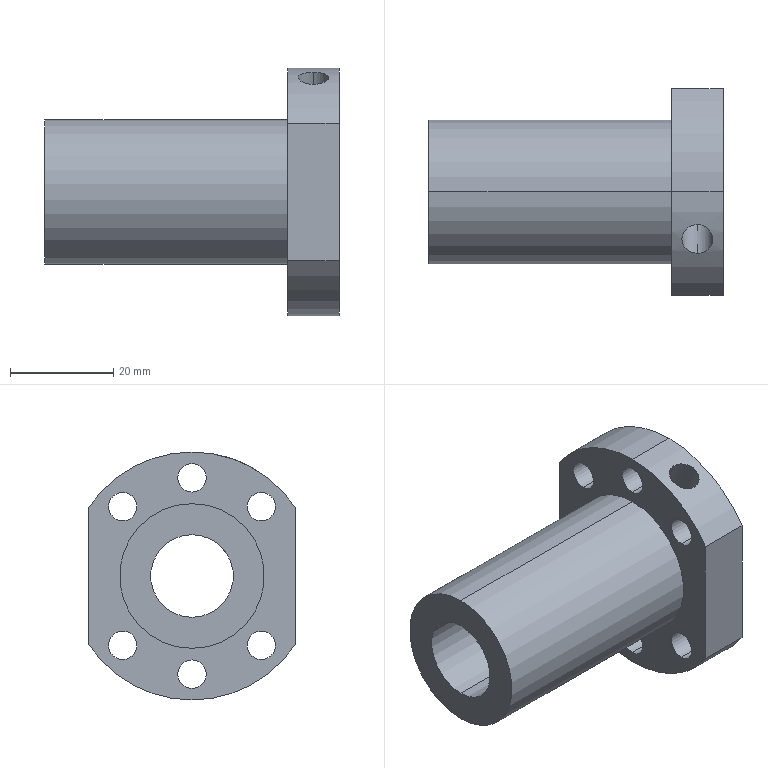Part | STEP file | Lead screw nut SFU01610-3V1.201001 | 1 solid | 26 faces | box 57 x 40 x 48 mm | volume 32254 mm3 | cylinder 21 | plane 5 | commonest cylinder face diameters 5.5 x12 48 x3 6 x2 16 x2 28 x2